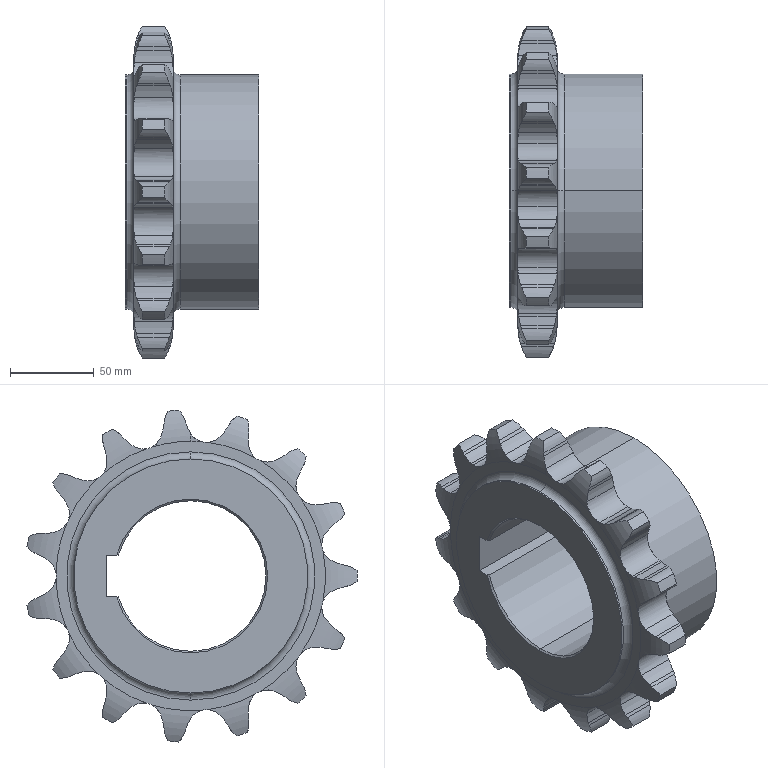Part | SolidWorks | features BaseBody 1 | 1 solid | 183 faces | box 80 x 197.46 x 198.492 mm | volume 920770 mm3 | cylinder 104 | plane 37 | torus 36 | cone 6 | commonest cylinder face diameters 32.838 x32 58.009 x31 22.441 x19 199 x15 140 x4 90 x3